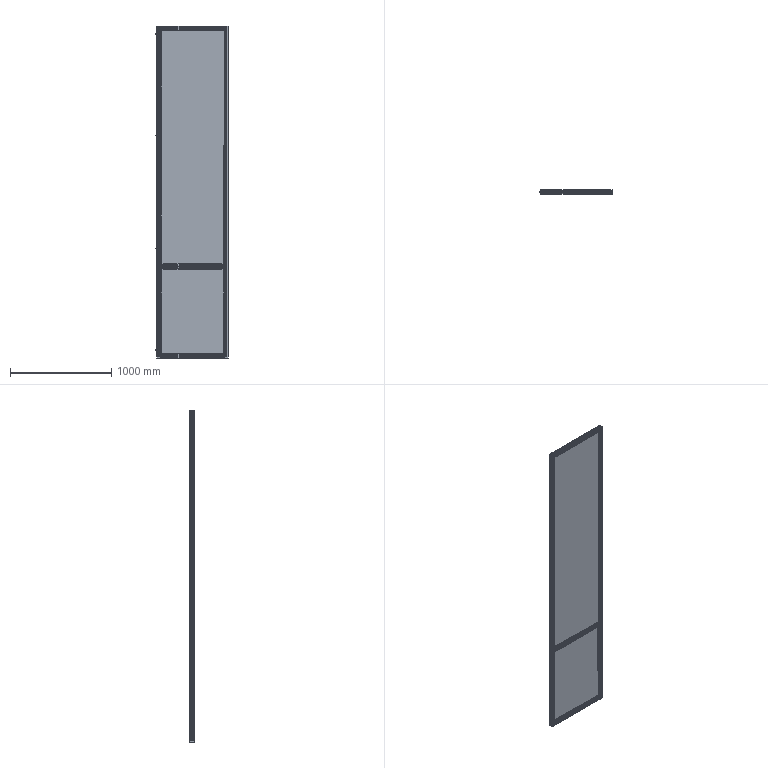Part | SolidWorks | features ReferencePattern 12, LocalLPattern 4 | 31 solids | 1970 faces | box 720.4 x 40 x 3280 mm | volume 15751167 mm3 | plane 1295 | cylinder 623 | cone 44 | spline 8 | commonest cylinder face diameters 5 x104 6.8 x103 2 x54 19 x36 6.6 x32 11 x32